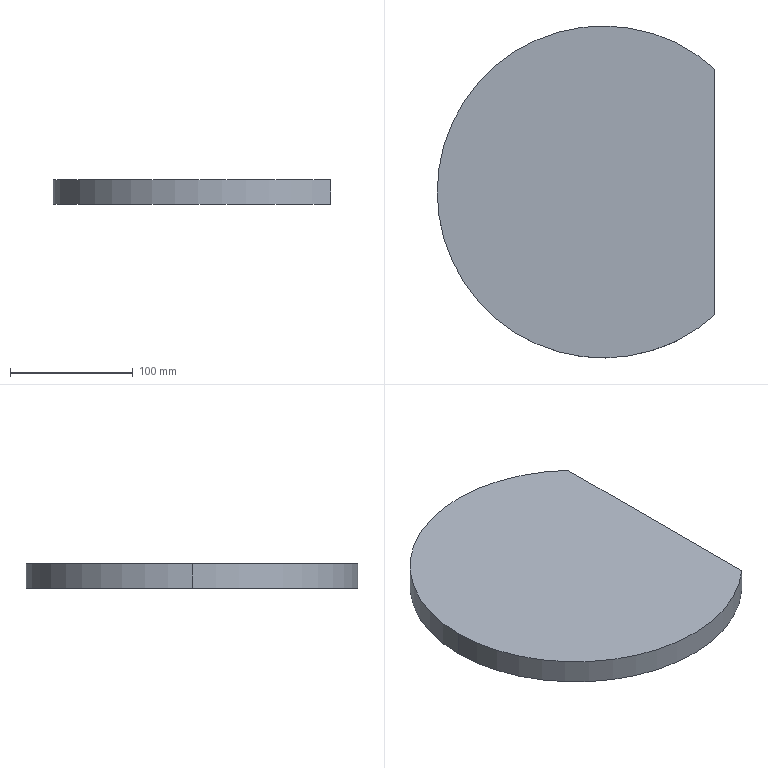Part | SolidWorks | features Extrusion 1 | 1 solid | 5 faces | box 225.69 x 270 x 20 mm | volume 1022431 mm3 | plane 3 | cylinder 2 | commonest cylinder face diameters 270 x2
STEP:
#1=CARTESIAN_POINT('',(-135.,0.,20.));
#2=VERTEX_POINT('',#1);
#3=CARTESIAN_POINT('',(90.69,-100.002,20.));
#4=VERTEX_POINT('',#3);
#5=CARTESIAN_POINT('',(0.,0.,20.));
#6=DIRECTION('',(0.,0.,1.));
#7=DIRECTION('',(1.,0.,0.));
#8=AXIS2_PLACEMENT_3D('',#5,#6,#7);
#9=CIRCLE('',#8,135.);
#10=EDGE_CURVE('',#2,#4,#9,.T.);
#11=ORIENTED_EDGE('',*,*,#10,.F.);
#12=CARTESIAN_POINT('',(-135.,0.,0.));
#13=VERTEX_POINT('',#12);
#14=CARTESIAN_POINT('',(-135.,0.,20.));
#15=DIRECTION('',(0.,0.,-1.));
#16=VECTOR('',#15,1000.);
#17=LINE('',#14,#16);
#18=EDGE_CURVE('',#2,#13,#17,.T.);
#19=ORIENTED_EDGE('',*,*,#18,.T.);
#20=CARTESIAN_POINT('',(90.69,-100.002,0.));
#21=VERTEX_POINT('',#20);
#22=CARTESIAN_POINT('',(0.,0.,0.));
#23=DIRECTION('',(0.,0.,1.));
#24=DIRECTION('',(1.,0.,0.));
#25=AXIS2_PLACEMENT_3D('',#22,#23,#24);
#26=CIRCLE('',#25,135.);
#27=EDGE_CURVE('',#13,#21,#26,.T.);
#28=ORIENTED_EDGE('',*,*,#27,.T.);
#29=CARTESIAN_POINT('',(90.69,-100.002,20.));
#30=DIRECTION('',(0.,0.,-1.));
#31=VECTOR('',#30,1000.);
#32=LINE('',#29,#31);
#33=EDGE_CURVE('',#4,#21,#32,.T.);
#34=ORIENTED_EDGE('',*,*,#33,.F.);
#35=EDGE_LOOP('',(#11,#19,#28,#34));
#36=FACE_OUTER_BOUND('',#35,.T.);
#37=CARTESIAN_POINT('',(0.,0.,20.));
#38=DIRECTION('',(0.,0.,-1.));
#39=DIRECTION('',(-1.,0.,0.));
#40=AXIS2_PLACEMENT_3D('',#37,#38,#39);
#41=CYLINDRICAL_SURFACE('',#40,135.);
#42=ADVANCED_FACE('',(#36),#41,.T.);
#43=ORIENTED_EDGE('',*,*,#18,.F.);
#44=CARTESIAN_POINT('',(90.69,100.002,20.));
#45=VERTEX_POINT('',#44);
#46=CARTESIAN_POINT('',(0.,0.,20.));
#47=DIRECTION('',(0.,0.,1.));
#48=DIRECTION('',(1.,0.,0.));
#49=AXIS2_PLACEMENT_3D('',#46,#47,#48);
#50=CIRCLE('',#49,135.);
#51=EDGE_CURVE('',#45,#2,#50,.T.);
#52=ORIENTED_EDGE('',*,*,#51,.F.);
#53=CARTESIAN_POINT('',(90.69,100.002,0.));
#54=VERTEX_POINT('',#53);
#55=CARTESIAN_POINT('',(90.69,100.002,20.));
#56=DIRECTION('',(0.,0.,-1.));
#57=VECTOR('',#56,1000.);
#58=LINE('',#55,#57);
#59=EDGE_CURVE('',#45,#54,#58,.T.);
#60=ORIENTED_EDGE('',*,*,#59,.T.);
#61=CARTESIAN_POINT('',(0.,0.,0.));
#62=DIRECTION('',(0.,0.,1.));
#63=DIRECTION('',(1.,0.,0.));
#64=AXIS2_PLACEMENT_3D('',#61,#62,#63);
#65=CIRCLE('',#64,135.);
#66=EDGE_CURVE('',#54,#13,#65,.T.);
#67=ORIENTED_EDGE('',*,*,#66,.T.);
#68=EDGE_LOOP('',(#43,#52,#60,#67));
#69=FACE_OUTER_BOUND('',#68,.T.);
#70=CARTESIAN_POINT('',(0.,0.,20.));
#71=DIRECTION('',(0.,0.,-1.));
#72=DIRECTION('',(-1.,0.,0.));
#73=AXIS2_PLACEMENT_3D('',#70,#71,#72);
#74=CYLINDRICAL_SURFACE('',#73,135.);
#75=ADVANCED_FACE('',(#69),#74,.T.);
#76=CARTESIAN_POINT('',(90.69,100.002,0.));
#77=DIRECTION('',(0.,1.,0.));
#78=VECTOR('',#77,1000.);
#79=LINE('',#76,#78);
#80=EDGE_CURVE('',#21,#54,#79,.T.);
#81=ORIENTED_EDGE('',*,*,#80,.T.);
#82=ORIENTED_EDGE('',*,*,#59,.F.);
#83=CARTESIAN_POINT('',(90.69,100.002,20.));
#84=DIRECTION('',(0.,1.,0.));
#85=VECTOR('',#84,1000.);
#86=LINE('',#83,#85);
#87=EDGE_CURVE('',#4,#45,#86,.T.);
#88=ORIENTED_EDGE('',*,*,#87,.F.);
#89=ORIENTED_EDGE('',*,*,#33,.T.);
#90=EDGE_LOOP('',(#81,#82,#88,#89));
#91=FACE_OUTER_BOUND('',#90,.T.);
#92=CARTESIAN_POINT('',(90.69,100.002,20.));
#93=DIRECTION('',(-1.,0.,0.));
#94=DIRECTION('',(0.,0.,1.));
#95=AXIS2_PLACEMENT_3D('',#92,#93,#94);
#96=PLANE('',#95);
#97=ADVANCED_FACE('',(#91),#96,.F.);
#98=ORIENTED_EDGE('',*,*,#51,.T.);
#99=ORIENTED_EDGE('',*,*,#10,.T.);
#100=ORIENTED_EDGE('',*,*,#87,.T.);
#101=EDGE_LOOP('',(#98,#99,#100));
#102=FACE_OUTER_BOUND('',#101,.T.);
#103=CARTESIAN_POINT('',(0.,0.,20.));
#104=DIRECTION('',(0.,0.,1.));
#105=DIRECTION('',(1.,0.,0.));
#106=AXIS2_PLACEMENT_3D('',#103,#104,#105);
#107=PLANE('',#106);
#108=ADVANCED_FACE('',(#102),#107,.T.);
#109=ORIENTED_EDGE('',*,*,#66,.F.);
#110=ORIENTED_EDGE('',*,*,#80,.F.);
#111=ORIENTED_EDGE('',*,*,#27,.F.);
#112=EDGE_LOOP('',(#109,#110,#111));
#113=FACE_OUTER_BOUND('',#112,.T.);
#114=CARTESIAN_POINT('',(0.,0.,0.));
#115=DIRECTION('',(0.,0.,1.));
#116=DIRECTION('',(1.,0.,0.));
#117=AXIS2_PLACEMENT_3D('',#114,#115,#116);
#118=PLANE('',#117);
#119=ADVANCED_FACE('',(#113),#118,.F.);
#120=CLOSED_SHELL('',(#42,#75,#97,#108,#119));
#121=MANIFOLD_SOLID_BREP('',#120);
#122=CARTESIAN_POINT('',(0.,0.,0.));
#123=DIRECTION('',(0.,0.,1.));
#124=DIRECTION('',(1.,0.,0.));
#125=AXIS2_PLACEMENT_3D('',#122,#123,#124);
#126=(LENGTH_UNIT()NAMED_UNIT(*)SI_UNIT(.MILLI.,.METRE.));
#127=UNCERTAINTY_MEASURE_WITH_UNIT(LENGTH_MEASURE(0.00001),#126,'','');
#128=(NAMED_UNIT(*)PLANE_ANGLE_UNIT()SI_UNIT($,.RADIAN.));
#129=(NAMED_UNIT(*)SI_UNIT($,.STERADIAN.)SOLID_ANGLE_UNIT());
#130=(GEOMETRIC_REPRESENTATION_CONTEXT(3)GLOBAL_UNCERTAINTY_ASSIGNED_CONTEXT((#127))GLOBAL_UNIT_ASSIGNED_CONTEXT((#126,#128,#129))REPRESENTATION_CONTEXT('',''));
#131=ADVANCED_BREP_SHAPE_REPRESENTATION('',(#121,#125),#130);